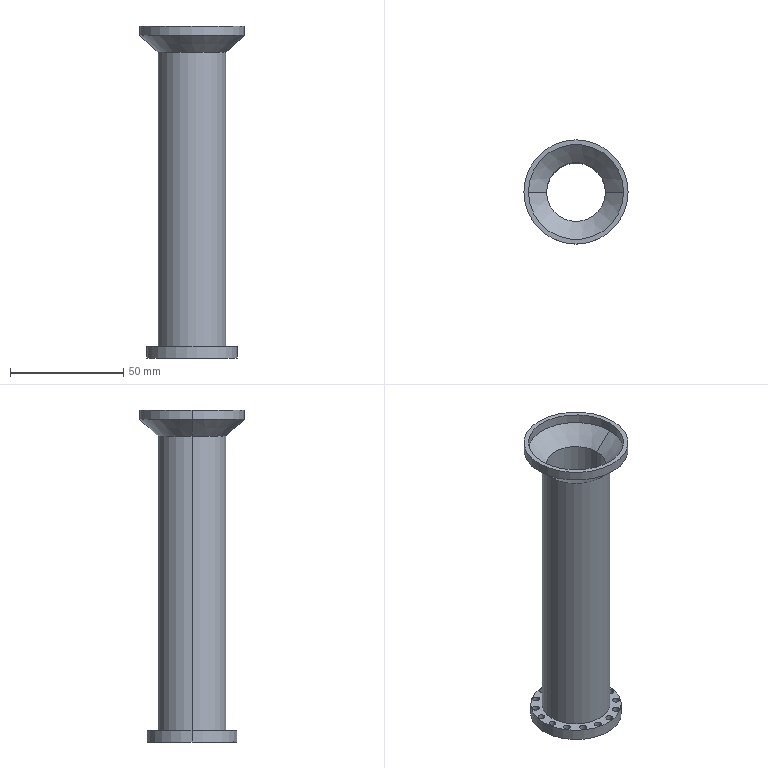Part | SolidWorks | features Cut 3, Extrusion 1, ICE 1, Revolution 1 | 2 solids | 51 faces | box 46 x 46 x 146.519 mm | volume 28748 mm3 | cylinder 42 | plane 5 | cone 4 | commonest cylinder face diameters 3 x32 26 x2 30 x2 40 x2 42 x2 46 x2